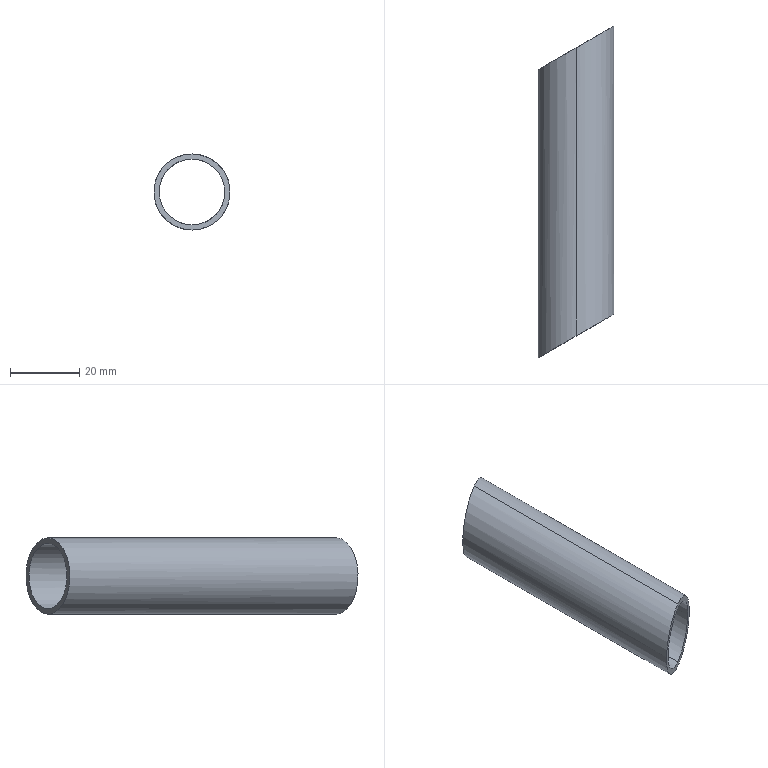Part | SolidWorks | features Extrusion 1, ICE 1 | 1 solid | 6 faces | box 22 x 96 x 22 mm | volume 8046 mm3 | cylinder 4 | plane 2 | commonest cylinder face diameters 19 x2 22 x2
STEP:
#1=CARTESIAN_POINT('',(0.,41.649,9.5));
#2=VERTEX_POINT('',#1);
#3=CARTESIAN_POINT('',(0.,41.649,-9.5));
#4=VERTEX_POINT('',#3);
#5=CARTESIAN_POINT('',(0.,41.649,9.5));
#6=CARTESIAN_POINT('',(-19.,30.679,9.5));
#7=CARTESIAN_POINT('',(-19.,30.679,-9.5));
#8=CARTESIAN_POINT('',(0.,41.649,-9.5));
#9=(BOUNDED_CURVE()B_SPLINE_CURVE(3,(#5,#6,#7,#8),.UNSPECIFIED.,.F.,.T.)B_SPLINE_CURVE_WITH_KNOTS((4,4),(4.712,7.854),.UNSPECIFIED.)CURVE()GEOMETRIC_REPRESENTATION_ITEM()RATIONAL_B_SPLINE_CURVE((1.,0.3333,0.3333,1.))REPRESENTATION_ITEM(''));
#10=EDGE_CURVE('',#2,#4,#9,.T.);
#11=ORIENTED_EDGE('',*,*,#10,.F.);
#12=CARTESIAN_POINT('',(0.,-41.649,9.5));
#13=VERTEX_POINT('',#12);
#14=CARTESIAN_POINT('',(0.,48.,9.5));
#15=DIRECTION('',(0.,-1.,0.));
#16=VECTOR('',#15,1000.);
#17=LINE('',#14,#16);
#18=EDGE_CURVE('',#2,#13,#17,.T.);
#19=ORIENTED_EDGE('',*,*,#18,.T.);
#20=CARTESIAN_POINT('',(0.,-41.649,-9.5));
#21=VERTEX_POINT('',#20);
#22=CARTESIAN_POINT('',(0.,-41.649,-9.5));
#23=CARTESIAN_POINT('',(-19.,-52.619,-9.5));
#24=CARTESIAN_POINT('',(-19.,-52.619,9.5));
#25=CARTESIAN_POINT('',(0.,-41.649,9.5));
#26=(BOUNDED_CURVE()B_SPLINE_CURVE(3,(#22,#23,#24,#25),.UNSPECIFIED.,.F.,.F.)B_SPLINE_CURVE_WITH_KNOTS((4,4),(4.712,7.854),.UNSPECIFIED.)CURVE()GEOMETRIC_REPRESENTATION_ITEM()RATIONAL_B_SPLINE_CURVE((1.,0.3333,0.3333,1.))REPRESENTATION_ITEM(''));
#27=EDGE_CURVE('',#21,#13,#26,.T.);
#28=ORIENTED_EDGE('',*,*,#27,.F.);
#29=CARTESIAN_POINT('',(0.,48.,-9.5));
#30=DIRECTION('',(0.,-1.,0.));
#31=VECTOR('',#30,1000.);
#32=LINE('',#29,#31);
#33=EDGE_CURVE('',#4,#21,#32,.T.);
#34=ORIENTED_EDGE('',*,*,#33,.F.);
#35=EDGE_LOOP('',(#11,#19,#28,#34));
#36=FACE_OUTER_BOUND('',#35,.T.);
#37=CARTESIAN_POINT('',(0.,48.,0.));
#38=DIRECTION('',(0.,-1.,0.));
#39=DIRECTION('',(0.,0.,-1.));
#40=AXIS2_PLACEMENT_3D('',#37,#38,#39);
#41=CYLINDRICAL_SURFACE('',#40,9.5);
#42=ADVANCED_FACE('',(#36),#41,.F.);
#43=CARTESIAN_POINT('',(0.,41.649,-11.));
#44=VERTEX_POINT('',#43);
#45=CARTESIAN_POINT('',(0.,41.649,11.));
#46=VERTEX_POINT('',#45);
#47=CARTESIAN_POINT('',(0.,41.649,-11.));
#48=CARTESIAN_POINT('',(22.,54.351,-11.));
#49=CARTESIAN_POINT('',(22.,54.351,11.));
#50=CARTESIAN_POINT('',(0.,41.649,11.));
#51=(BOUNDED_CURVE()B_SPLINE_CURVE(3,(#47,#48,#49,#50),.UNSPECIFIED.,.F.,.F.)B_SPLINE_CURVE_WITH_KNOTS((4,4),(1.571,4.712),.UNSPECIFIED.)CURVE()GEOMETRIC_REPRESENTATION_ITEM()RATIONAL_B_SPLINE_CURVE((1.,0.3333,0.3333,1.))REPRESENTATION_ITEM(''));
#52=EDGE_CURVE('',#44,#46,#51,.T.);
#53=ORIENTED_EDGE('',*,*,#52,.T.);
#54=CARTESIAN_POINT('',(0.,-41.649,11.));
#55=VERTEX_POINT('',#54);
#56=CARTESIAN_POINT('',(0.,48.,11.));
#57=DIRECTION('',(0.,-1.,0.));
#58=VECTOR('',#57,1000.);
#59=LINE('',#56,#58);
#60=EDGE_CURVE('',#46,#55,#59,.T.);
#61=ORIENTED_EDGE('',*,*,#60,.T.);
#62=CARTESIAN_POINT('',(0.,-41.649,-11.));
#63=VERTEX_POINT('',#62);
#64=CARTESIAN_POINT('',(0.,-41.649,11.));
#65=CARTESIAN_POINT('',(22.,-28.947,11.));
#66=CARTESIAN_POINT('',(22.,-28.947,-11.));
#67=CARTESIAN_POINT('',(0.,-41.649,-11.));
#68=(BOUNDED_CURVE()B_SPLINE_CURVE(3,(#64,#65,#66,#67),.UNSPECIFIED.,.F.,.T.)B_SPLINE_CURVE_WITH_KNOTS((4,4),(1.571,4.712),.UNSPECIFIED.)CURVE()GEOMETRIC_REPRESENTATION_ITEM()RATIONAL_B_SPLINE_CURVE((1.,0.3333,0.3333,1.))REPRESENTATION_ITEM(''));
#69=EDGE_CURVE('',#55,#63,#68,.T.);
#70=ORIENTED_EDGE('',*,*,#69,.T.);
#71=CARTESIAN_POINT('',(0.,48.,-11.));
#72=DIRECTION('',(0.,-1.,0.));
#73=VECTOR('',#72,1000.);
#74=LINE('',#71,#73);
#75=EDGE_CURVE('',#44,#63,#74,.T.);
#76=ORIENTED_EDGE('',*,*,#75,.F.);
#77=EDGE_LOOP('',(#53,#61,#70,#76));
#78=FACE_OUTER_BOUND('',#77,.T.);
#79=CARTESIAN_POINT('',(0.,48.,0.));
#80=DIRECTION('',(0.,-1.,0.));
#81=DIRECTION('',(0.,0.,-1.));
#82=AXIS2_PLACEMENT_3D('',#79,#80,#81);
#83=CYLINDRICAL_SURFACE('',#82,11.);
#84=ADVANCED_FACE('',(#78),#83,.T.);
#85=ORIENTED_EDGE('',*,*,#60,.F.);
#86=CARTESIAN_POINT('',(0.,41.649,11.));
#87=CARTESIAN_POINT('',(-22.,28.947,11.));
#88=CARTESIAN_POINT('',(-22.,28.947,-11.));
#89=CARTESIAN_POINT('',(0.,41.649,-11.));
#90=(BOUNDED_CURVE()B_SPLINE_CURVE(3,(#86,#87,#88,#89),.UNSPECIFIED.,.F.,.F.)B_SPLINE_CURVE_WITH_KNOTS((4,4),(4.712,7.854),.UNSPECIFIED.)CURVE()GEOMETRIC_REPRESENTATION_ITEM()RATIONAL_B_SPLINE_CURVE((1.,0.3333,0.3333,1.))REPRESENTATION_ITEM(''));
#91=EDGE_CURVE('',#46,#44,#90,.T.);
#92=ORIENTED_EDGE('',*,*,#91,.T.);
#93=ORIENTED_EDGE('',*,*,#75,.T.);
#94=CARTESIAN_POINT('',(0.,-41.649,-11.));
#95=CARTESIAN_POINT('',(-22.,-54.351,-11.));
#96=CARTESIAN_POINT('',(-22.,-54.351,11.));
#97=CARTESIAN_POINT('',(0.,-41.649,11.));
#98=(BOUNDED_CURVE()B_SPLINE_CURVE(3,(#94,#95,#96,#97),.UNSPECIFIED.,.F.,.F.)B_SPLINE_CURVE_WITH_KNOTS((4,4),(4.712,7.854),.UNSPECIFIED.)CURVE()GEOMETRIC_REPRESENTATION_ITEM()RATIONAL_B_SPLINE_CURVE((1.,0.3333,0.3333,1.))REPRESENTATION_ITEM(''));
#99=EDGE_CURVE('',#63,#55,#98,.T.);
#100=ORIENTED_EDGE('',*,*,#99,.T.);
#101=EDGE_LOOP('',(#85,#92,#93,#100));
#102=FACE_OUTER_BOUND('',#101,.T.);
#103=CARTESIAN_POINT('',(0.,48.,0.));
#104=DIRECTION('',(0.,-1.,0.));
#105=DIRECTION('',(0.,0.,-1.));
#106=AXIS2_PLACEMENT_3D('',#103,#104,#105);
#107=CYLINDRICAL_SURFACE('',#106,11.);
#108=ADVANCED_FACE('',(#102),#107,.T.);
#109=ORIENTED_EDGE('',*,*,#18,.F.);
#110=CARTESIAN_POINT('',(0.,41.649,-9.5));
#111=CARTESIAN_POINT('',(19.,52.619,-9.5));
#112=CARTESIAN_POINT('',(19.,52.619,9.5));
#113=CARTESIAN_POINT('',(0.,41.649,9.5));
#114=(BOUNDED_CURVE()B_SPLINE_CURVE(3,(#110,#111,#112,#113),.UNSPECIFIED.,.F.,.F.)B_SPLINE_CURVE_WITH_KNOTS((4,4),(1.571,4.712),.UNSPECIFIED.)CURVE()GEOMETRIC_REPRESENTATION_ITEM()RATIONAL_B_SPLINE_CURVE((1.,0.3333,0.3333,1.))REPRESENTATION_ITEM(''));
#115=EDGE_CURVE('',#4,#2,#114,.T.);
#116=ORIENTED_EDGE('',*,*,#115,.F.);
#117=ORIENTED_EDGE('',*,*,#33,.T.);
#118=CARTESIAN_POINT('',(0.,-41.649,9.5));
#119=CARTESIAN_POINT('',(19.,-30.679,9.5));
#120=CARTESIAN_POINT('',(19.,-30.679,-9.5));
#121=CARTESIAN_POINT('',(0.,-41.649,-9.5));
#122=(BOUNDED_CURVE()B_SPLINE_CURVE(3,(#118,#119,#120,#121),.UNSPECIFIED.,.F.,.T.)B_SPLINE_CURVE_WITH_KNOTS((4,4),(1.571,4.712),.UNSPECIFIED.)CURVE()GEOMETRIC_REPRESENTATION_ITEM()RATIONAL_B_SPLINE_CURVE((1.,0.3333,0.3333,1.))REPRESENTATION_ITEM(''));
#123=EDGE_CURVE('',#13,#21,#122,.T.);
#124=ORIENTED_EDGE('',*,*,#123,.F.);
#125=EDGE_LOOP('',(#109,#116,#117,#124));
#126=FACE_OUTER_BOUND('',#125,.T.);
#127=CARTESIAN_POINT('',(0.,48.,0.));
#128=DIRECTION('',(0.,-1.,0.));
#129=DIRECTION('',(0.,0.,-1.));
#130=AXIS2_PLACEMENT_3D('',#127,#128,#129);
#131=CYLINDRICAL_SURFACE('',#130,9.5);
#132=ADVANCED_FACE('',(#126),#131,.F.);
#133=ORIENTED_EDGE('',*,*,#115,.T.);
#134=ORIENTED_EDGE('',*,*,#10,.T.);
#135=EDGE_LOOP('',(#133,#134));
#136=FACE_BOUND('',#135,.T.);
#137=ORIENTED_EDGE('',*,*,#52,.F.);
#138=ORIENTED_EDGE('',*,*,#91,.F.);
#139=EDGE_LOOP('',(#137,#138));
#140=FACE_OUTER_BOUND('',#139,.T.);
#141=CARTESIAN_POINT('',(-11.,35.298,-11.));
#142=DIRECTION('',(0.5,-0.866,0.));
#143=DIRECTION('',(0.866,0.5,0.));
#144=AXIS2_PLACEMENT_3D('',#141,#142,#143);
#145=PLANE('',#144);
#146=ADVANCED_FACE('',(#136,#140),#145,.F.);
#147=ORIENTED_EDGE('',*,*,#27,.T.);
#148=ORIENTED_EDGE('',*,*,#123,.T.);
#149=EDGE_LOOP('',(#147,#148));
#150=FACE_BOUND('',#149,.T.);
#151=ORIENTED_EDGE('',*,*,#99,.F.);
#152=ORIENTED_EDGE('',*,*,#69,.F.);
#153=EDGE_LOOP('',(#151,#152));
#154=FACE_OUTER_BOUND('',#153,.T.);
#155=CARTESIAN_POINT('',(-11.,-48.,-11.));
#156=DIRECTION('',(-0.5,0.866,0.));
#157=DIRECTION('',(-0.866,-0.5,0.));
#158=AXIS2_PLACEMENT_3D('',#155,#156,#157);
#159=PLANE('',#158);
#160=ADVANCED_FACE('',(#150,#154),#159,.F.);
#161=CLOSED_SHELL('',(#42,#84,#108,#132,#146,#160));
#162=MANIFOLD_SOLID_BREP('',#161);
#163=CARTESIAN_POINT('',(0.,0.,0.));
#164=DIRECTION('',(0.,0.,1.));
#165=DIRECTION('',(1.,0.,0.));
#166=AXIS2_PLACEMENT_3D('',#163,#164,#165);
#167=(LENGTH_UNIT()NAMED_UNIT(*)SI_UNIT(.MILLI.,.METRE.));
#168=UNCERTAINTY_MEASURE_WITH_UNIT(LENGTH_MEASURE(0.00001),#167,'','');
#169=(NAMED_UNIT(*)PLANE_ANGLE_UNIT()SI_UNIT($,.RADIAN.));
#170=(NAMED_UNIT(*)SI_UNIT($,.STERADIAN.)SOLID_ANGLE_UNIT());
#171=(GEOMETRIC_REPRESENTATION_CONTEXT(3)GLOBAL_UNCERTAINTY_ASSIGNED_CONTEXT((#168))GLOBAL_UNIT_ASSIGNED_CONTEXT((#167,#169,#170))REPRESENTATION_CONTEXT('',''));
#172=ADVANCED_BREP_SHAPE_REPRESENTATION('',(#162,#166),#171);